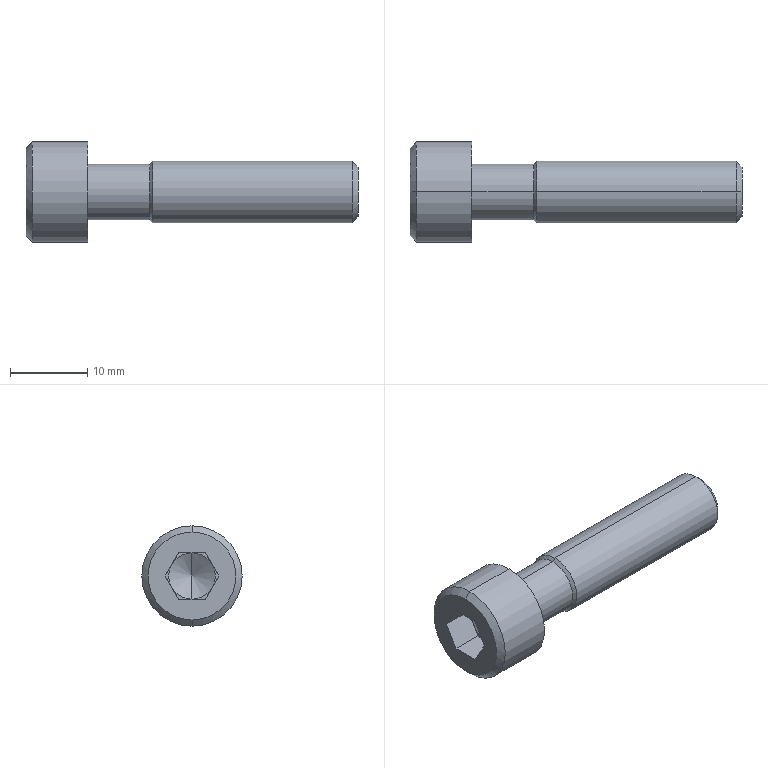Part | STEP file | 0244_Z_018_SCBS8-35_1 | 1 solid | 29 faces | box 43 x 13 x 13 mm | volume 2585 mm3 | plane 15 | cone 8 | cylinder 6 | commonest cylinder face diameters 7.232 x2 8 x2 13 x2